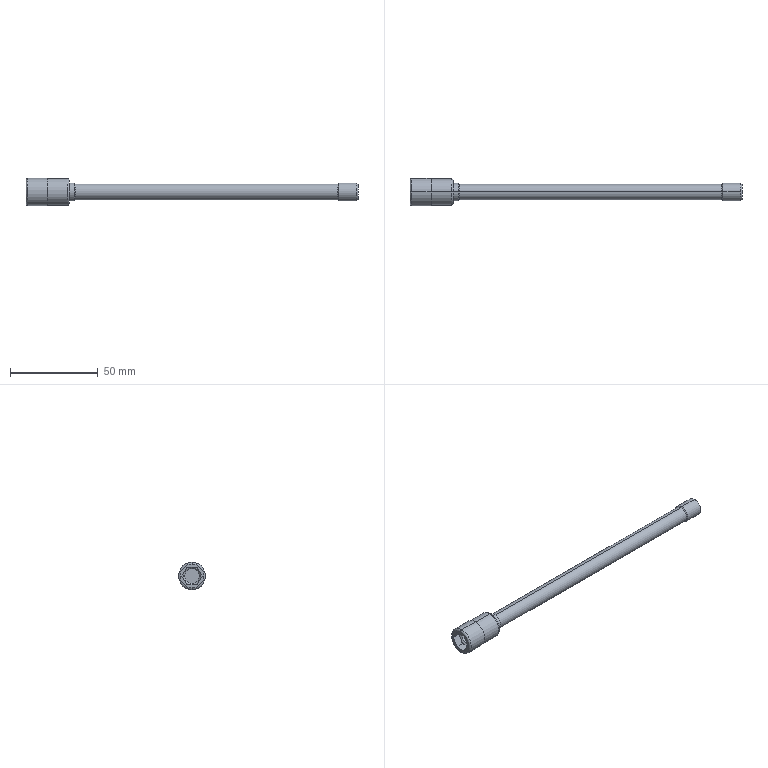Part | STEP file | SCT80_1007 | 1 solid | 41 faces | box 189 x 15.5 x 15.5 mm | volume 13853 mm3 | plane 17 | cylinder 12 | cone 8 | torus 4 | commonest cylinder face diameters 10 x4 8.376 x2 8.9 x2 15 x2 15.5 x2